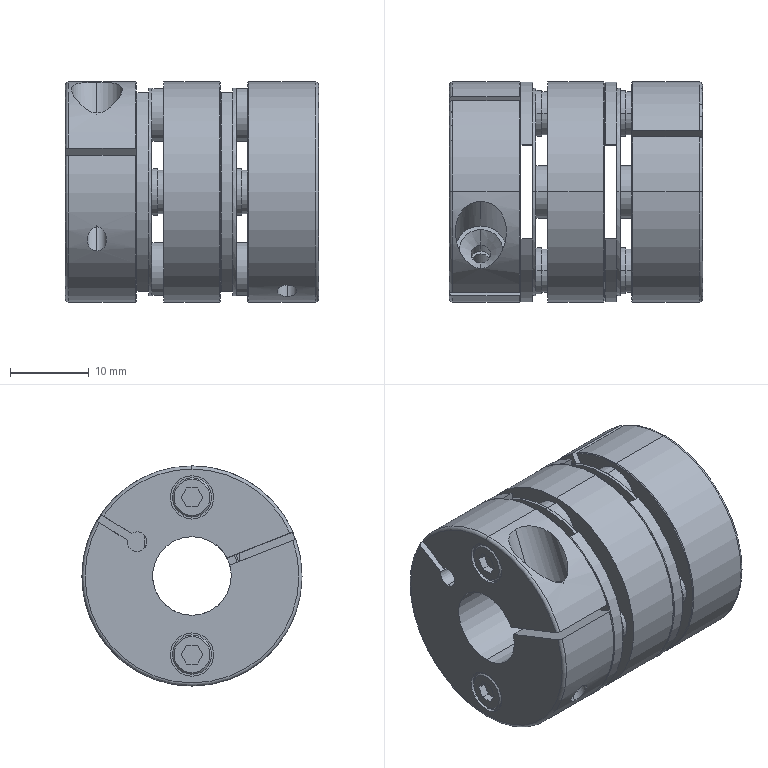Part | STEP file | Guide wheel mechanism revised.sldasm-Part-356 | 1 solid | 197 faces | box 32.2 x 28 x 28 mm | volume 14007 mm3 | cylinder 87 | plane 78 | cone 25 | torus 7 | commonest cylinder face diameters 5.5 x16 28 x13 2.459 x8 5 x8 5.9 x8 6.7 x8